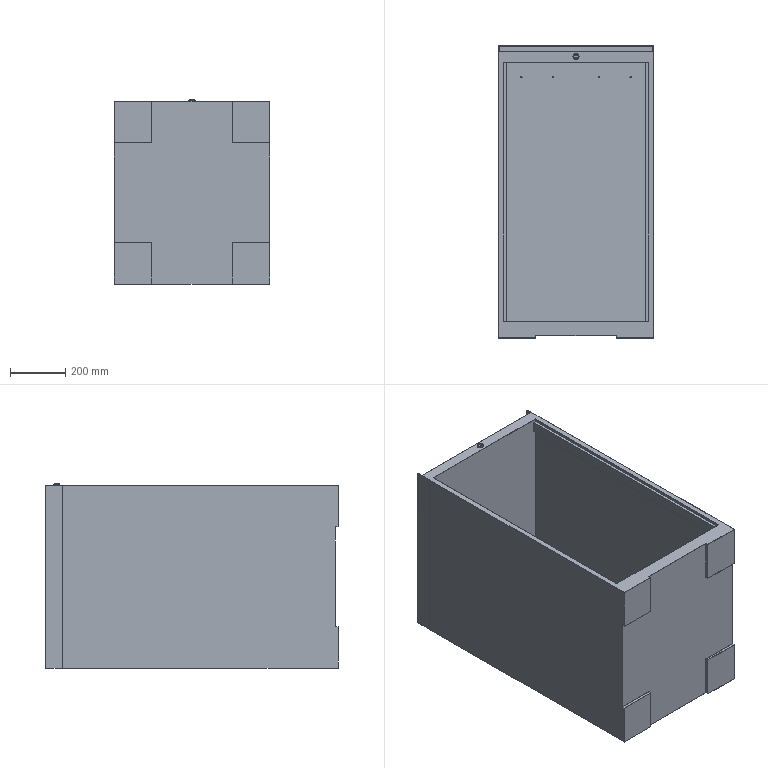Part | SolidWorks | features ICE 10, Fillet 2, Extrusion 1, HoleWzd 1 | 1 solid | 192 faces | box 560 x 1055 x 665 mm | volume 61823880 mm3 | cylinder 86 | plane 60 | torus 24 | sphere 20 | cone 2 | commonest cylinder face diameters 1 x70 5 x8 2 x2 15.5 x2 16 x2 22 x2